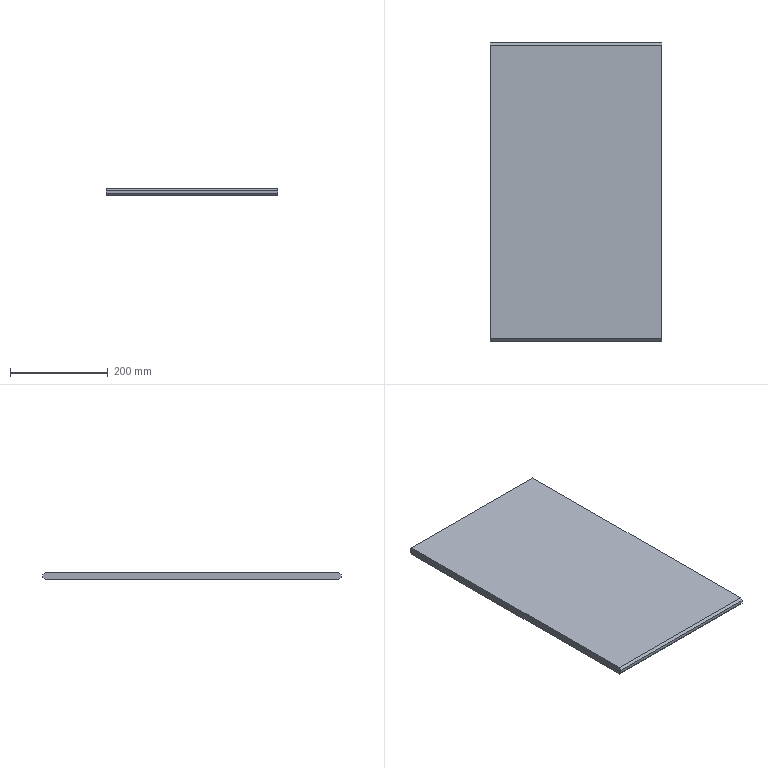Part | SolidWorks | features Chamfer 1, Extrusion 1 | 1 solid | 10 faces | box 350 x 610 x 16 mm | volume 3398500 mm3 | plane 10
STEP:
#1=CARTESIAN_POINT('',(0.,610.,11.));
#2=VERTEX_POINT('',#1);
#3=CARTESIAN_POINT('',(0.,610.,5.));
#4=VERTEX_POINT('',#3);
#5=CARTESIAN_POINT('',(0.,610.,16.));
#6=DIRECTION('',(0.,0.,-1.));
#7=VECTOR('',#6,1000.);
#8=LINE('',#5,#7);
#9=EDGE_CURVE('',#2,#4,#8,.T.);
#10=ORIENTED_EDGE('',*,*,#9,.T.);
#11=CARTESIAN_POINT('',(0.,605.,0.));
#12=VERTEX_POINT('',#11);
#13=CARTESIAN_POINT('',(0.,610.,5.));
#14=DIRECTION('',(0.,-0.7071,-0.7071));
#15=VECTOR('',#14,1000.);
#16=LINE('',#13,#15);
#17=EDGE_CURVE('',#4,#12,#16,.T.);
#18=ORIENTED_EDGE('',*,*,#17,.T.);
#19=CARTESIAN_POINT('',(0.,5.,0.));
#20=VERTEX_POINT('',#19);
#21=CARTESIAN_POINT('',(0.,0.,0.));
#22=DIRECTION('',(0.,-1.,0.));
#23=VECTOR('',#22,1000.);
#24=LINE('',#21,#23);
#25=EDGE_CURVE('',#12,#20,#24,.T.);
#26=ORIENTED_EDGE('',*,*,#25,.T.);
#27=CARTESIAN_POINT('',(0.,0.,5.));
#28=VERTEX_POINT('',#27);
#29=CARTESIAN_POINT('',(0.,0.,5.));
#30=DIRECTION('',(0.,-0.7071,0.7071));
#31=VECTOR('',#30,1000.);
#32=LINE('',#29,#31);
#33=EDGE_CURVE('',#20,#28,#32,.T.);
#34=ORIENTED_EDGE('',*,*,#33,.T.);
#35=CARTESIAN_POINT('',(0.,0.,11.));
#36=VERTEX_POINT('',#35);
#37=CARTESIAN_POINT('',(0.,0.,16.));
#38=DIRECTION('',(0.,0.,-1.));
#39=VECTOR('',#38,1000.);
#40=LINE('',#37,#39);
#41=EDGE_CURVE('',#36,#28,#40,.T.);
#42=ORIENTED_EDGE('',*,*,#41,.F.);
#43=CARTESIAN_POINT('',(0.,5.,16.));
#44=VERTEX_POINT('',#43);
#45=CARTESIAN_POINT('',(0.,5.,16.));
#46=DIRECTION('',(0.,0.7071,0.7071));
#47=VECTOR('',#46,1000.);
#48=LINE('',#45,#47);
#49=EDGE_CURVE('',#36,#44,#48,.T.);
#50=ORIENTED_EDGE('',*,*,#49,.T.);
#51=CARTESIAN_POINT('',(0.,605.,16.));
#52=VERTEX_POINT('',#51);
#53=CARTESIAN_POINT('',(0.,0.,16.));
#54=DIRECTION('',(0.,-1.,0.));
#55=VECTOR('',#54,1000.);
#56=LINE('',#53,#55);
#57=EDGE_CURVE('',#52,#44,#56,.T.);
#58=ORIENTED_EDGE('',*,*,#57,.F.);
#59=CARTESIAN_POINT('',(0.,605.,16.));
#60=DIRECTION('',(0.,0.7071,-0.7071));
#61=VECTOR('',#60,1000.);
#62=LINE('',#59,#61);
#63=EDGE_CURVE('',#52,#2,#62,.T.);
#64=ORIENTED_EDGE('',*,*,#63,.T.);
#65=EDGE_LOOP('',(#10,#18,#26,#34,#42,#50,#58,#64));
#66=FACE_OUTER_BOUND('',#65,.T.);
#67=CARTESIAN_POINT('',(0.,0.,16.));
#68=DIRECTION('',(1.,0.,0.));
#69=DIRECTION('',(0.,0.,-1.));
#70=AXIS2_PLACEMENT_3D('',#67,#68,#69);
#71=PLANE('',#70);
#72=ADVANCED_FACE('',(#66),#71,.F.);
#73=ORIENTED_EDGE('',*,*,#41,.T.);
#74=CARTESIAN_POINT('',(350.,0.,5.));
#75=VERTEX_POINT('',#74);
#76=CARTESIAN_POINT('',(350.,0.,5.));
#77=DIRECTION('',(1.,0.,0.));
#78=VECTOR('',#77,1000.);
#79=LINE('',#76,#78);
#80=EDGE_CURVE('',#28,#75,#79,.T.);
#81=ORIENTED_EDGE('',*,*,#80,.T.);
#82=CARTESIAN_POINT('',(350.,0.,11.));
#83=VERTEX_POINT('',#82);
#84=CARTESIAN_POINT('',(350.,0.,16.));
#85=DIRECTION('',(0.,0.,-1.));
#86=VECTOR('',#85,1000.);
#87=LINE('',#84,#86);
#88=EDGE_CURVE('',#83,#75,#87,.T.);
#89=ORIENTED_EDGE('',*,*,#88,.F.);
#90=CARTESIAN_POINT('',(0.,0.,11.));
#91=DIRECTION('',(-1.,0.,0.));
#92=VECTOR('',#91,1000.);
#93=LINE('',#90,#92);
#94=EDGE_CURVE('',#83,#36,#93,.T.);
#95=ORIENTED_EDGE('',*,*,#94,.T.);
#96=EDGE_LOOP('',(#73,#81,#89,#95));
#97=FACE_OUTER_BOUND('',#96,.T.);
#98=CARTESIAN_POINT('',(0.,0.,16.));
#99=DIRECTION('',(0.,1.,0.));
#100=DIRECTION('',(0.,0.,1.));
#101=AXIS2_PLACEMENT_3D('',#98,#99,#100);
#102=PLANE('',#101);
#103=ADVANCED_FACE('',(#97),#102,.F.);
#104=CARTESIAN_POINT('',(350.,5.,0.));
#105=VERTEX_POINT('',#104);
#106=CARTESIAN_POINT('',(350.,605.,0.));
#107=VERTEX_POINT('',#106);
#108=CARTESIAN_POINT('',(350.,0.,0.));
#109=DIRECTION('',(0.,1.,0.));
#110=VECTOR('',#109,1000.);
#111=LINE('',#108,#110);
#112=EDGE_CURVE('',#105,#107,#111,.T.);
#113=ORIENTED_EDGE('',*,*,#112,.T.);
#114=CARTESIAN_POINT('',(350.,610.,5.));
#115=VERTEX_POINT('',#114);
#116=CARTESIAN_POINT('',(350.,610.,5.));
#117=DIRECTION('',(0.,0.7071,0.7071));
#118=VECTOR('',#117,1000.);
#119=LINE('',#116,#118);
#120=EDGE_CURVE('',#107,#115,#119,.T.);
#121=ORIENTED_EDGE('',*,*,#120,.T.);
#122=CARTESIAN_POINT('',(350.,610.,11.));
#123=VERTEX_POINT('',#122);
#124=CARTESIAN_POINT('',(350.,610.,16.));
#125=DIRECTION('',(0.,0.,-1.));
#126=VECTOR('',#125,1000.);
#127=LINE('',#124,#126);
#128=EDGE_CURVE('',#123,#115,#127,.T.);
#129=ORIENTED_EDGE('',*,*,#128,.F.);
#130=CARTESIAN_POINT('',(350.,605.,16.));
#131=VERTEX_POINT('',#130);
#132=CARTESIAN_POINT('',(350.,605.,16.));
#133=DIRECTION('',(0.,-0.7071,0.7071));
#134=VECTOR('',#133,1000.);
#135=LINE('',#132,#134);
#136=EDGE_CURVE('',#123,#131,#135,.T.);
#137=ORIENTED_EDGE('',*,*,#136,.T.);
#138=CARTESIAN_POINT('',(350.,5.,16.));
#139=VERTEX_POINT('',#138);
#140=CARTESIAN_POINT('',(350.,0.,16.));
#141=DIRECTION('',(0.,1.,0.));
#142=VECTOR('',#141,1000.);
#143=LINE('',#140,#142);
#144=EDGE_CURVE('',#139,#131,#143,.T.);
#145=ORIENTED_EDGE('',*,*,#144,.F.);
#146=CARTESIAN_POINT('',(350.,5.,16.));
#147=DIRECTION('',(0.,-0.7071,-0.7071));
#148=VECTOR('',#147,1000.);
#149=LINE('',#146,#148);
#150=EDGE_CURVE('',#139,#83,#149,.T.);
#151=ORIENTED_EDGE('',*,*,#150,.T.);
#152=ORIENTED_EDGE('',*,*,#88,.T.);
#153=CARTESIAN_POINT('',(350.,0.,5.));
#154=DIRECTION('',(0.,0.7071,-0.7071));
#155=VECTOR('',#154,1000.);
#156=LINE('',#153,#155);
#157=EDGE_CURVE('',#75,#105,#156,.T.);
#158=ORIENTED_EDGE('',*,*,#157,.T.);
#159=EDGE_LOOP('',(#113,#121,#129,#137,#145,#151,#152,#158));
#160=FACE_OUTER_BOUND('',#159,.T.);
#161=CARTESIAN_POINT('',(350.,0.,16.));
#162=DIRECTION('',(-1.,0.,0.));
#163=DIRECTION('',(0.,0.,1.));
#164=AXIS2_PLACEMENT_3D('',#161,#162,#163);
#165=PLANE('',#164);
#166=ADVANCED_FACE('',(#160),#165,.F.);
#167=ORIENTED_EDGE('',*,*,#128,.T.);
#168=CARTESIAN_POINT('',(0.,610.,5.));
#169=DIRECTION('',(-1.,0.,0.));
#170=VECTOR('',#169,1000.);
#171=LINE('',#168,#170);
#172=EDGE_CURVE('',#115,#4,#171,.T.);
#173=ORIENTED_EDGE('',*,*,#172,.T.);
#174=ORIENTED_EDGE('',*,*,#9,.F.);
#175=CARTESIAN_POINT('',(0.,610.,11.));
#176=DIRECTION('',(1.,0.,0.));
#177=VECTOR('',#176,1000.);
#178=LINE('',#175,#177);
#179=EDGE_CURVE('',#2,#123,#178,.T.);
#180=ORIENTED_EDGE('',*,*,#179,.T.);
#181=EDGE_LOOP('',(#167,#173,#174,#180));
#182=FACE_OUTER_BOUND('',#181,.T.);
#183=CARTESIAN_POINT('',(0.,610.,16.));
#184=DIRECTION('',(0.,-1.,0.));
#185=DIRECTION('',(0.,0.,-1.));
#186=AXIS2_PLACEMENT_3D('',#183,#184,#185);
#187=PLANE('',#186);
#188=ADVANCED_FACE('',(#182),#187,.F.);
#189=ORIENTED_EDGE('',*,*,#144,.T.);
#190=CARTESIAN_POINT('',(0.,605.,16.));
#191=DIRECTION('',(-1.,0.,0.));
#192=VECTOR('',#191,1000.);
#193=LINE('',#190,#192);
#194=EDGE_CURVE('',#131,#52,#193,.T.);
#195=ORIENTED_EDGE('',*,*,#194,.T.);
#196=ORIENTED_EDGE('',*,*,#57,.T.);
#197=CARTESIAN_POINT('',(0.,5.,16.));
#198=DIRECTION('',(1.,0.,0.));
#199=VECTOR('',#198,1000.);
#200=LINE('',#197,#199);
#201=EDGE_CURVE('',#44,#139,#200,.T.);
#202=ORIENTED_EDGE('',*,*,#201,.T.);
#203=EDGE_LOOP('',(#189,#195,#196,#202));
#204=FACE_OUTER_BOUND('',#203,.T.);
#205=CARTESIAN_POINT('',(0.,610.,16.));
#206=DIRECTION('',(0.,0.,-1.));
#207=DIRECTION('',(-1.,0.,0.));
#208=AXIS2_PLACEMENT_3D('',#205,#206,#207);
#209=PLANE('',#208);
#210=ADVANCED_FACE('',(#204),#209,.F.);
#211=ORIENTED_EDGE('',*,*,#25,.F.);
#212=CARTESIAN_POINT('',(350.,605.,0.));
#213=DIRECTION('',(1.,0.,0.));
#214=VECTOR('',#213,1000.);
#215=LINE('',#212,#214);
#216=EDGE_CURVE('',#12,#107,#215,.T.);
#217=ORIENTED_EDGE('',*,*,#216,.T.);
#218=ORIENTED_EDGE('',*,*,#112,.F.);
#219=CARTESIAN_POINT('',(0.,5.,0.));
#220=DIRECTION('',(-1.,0.,0.));
#221=VECTOR('',#220,1000.);
#222=LINE('',#219,#221);
#223=EDGE_CURVE('',#105,#20,#222,.T.);
#224=ORIENTED_EDGE('',*,*,#223,.T.);
#225=EDGE_LOOP('',(#211,#217,#218,#224));
#226=FACE_OUTER_BOUND('',#225,.T.);
#227=CARTESIAN_POINT('',(0.,610.,0.));
#228=DIRECTION('',(0.,0.,-1.));
#229=DIRECTION('',(-1.,0.,0.));
#230=AXIS2_PLACEMENT_3D('',#227,#228,#229);
#231=PLANE('',#230);
#232=ADVANCED_FACE('',(#226),#231,.T.);
#233=ORIENTED_EDGE('',*,*,#120,.F.);
#234=ORIENTED_EDGE('',*,*,#216,.F.);
#235=ORIENTED_EDGE('',*,*,#17,.F.);
#236=ORIENTED_EDGE('',*,*,#172,.F.);
#237=EDGE_LOOP('',(#233,#234,#235,#236));
#238=FACE_OUTER_BOUND('',#237,.T.);
#239=CARTESIAN_POINT('',(0.,610.,5.));
#240=DIRECTION('',(0.,0.7071,-0.7071));
#241=DIRECTION('',(0.,0.7071,0.7071));
#242=AXIS2_PLACEMENT_3D('',#239,#240,#241);
#243=PLANE('',#242);
#244=ADVANCED_FACE('',(#238),#243,.T.);
#245=ORIENTED_EDGE('',*,*,#136,.F.);
#246=ORIENTED_EDGE('',*,*,#179,.F.);
#247=ORIENTED_EDGE('',*,*,#63,.F.);
#248=ORIENTED_EDGE('',*,*,#194,.F.);
#249=EDGE_LOOP('',(#245,#246,#247,#248));
#250=FACE_OUTER_BOUND('',#249,.T.);
#251=CARTESIAN_POINT('',(0.,605.,16.));
#252=DIRECTION('',(0.,-0.7071,-0.7071));
#253=DIRECTION('',(0.,0.7071,-0.7071));
#254=AXIS2_PLACEMENT_3D('',#251,#252,#253);
#255=PLANE('',#254);
#256=ADVANCED_FACE('',(#250),#255,.F.);
#257=ORIENTED_EDGE('',*,*,#33,.F.);
#258=ORIENTED_EDGE('',*,*,#223,.F.);
#259=ORIENTED_EDGE('',*,*,#157,.F.);
#260=ORIENTED_EDGE('',*,*,#80,.F.);
#261=EDGE_LOOP('',(#257,#258,#259,#260));
#262=FACE_OUTER_BOUND('',#261,.T.);
#263=CARTESIAN_POINT('',(0.,0.,5.));
#264=DIRECTION('',(0.,-0.7071,-0.7071));
#265=DIRECTION('',(0.,0.7071,-0.7071));
#266=AXIS2_PLACEMENT_3D('',#263,#264,#265);
#267=PLANE('',#266);
#268=ADVANCED_FACE('',(#262),#267,.T.);
#269=ORIENTED_EDGE('',*,*,#49,.F.);
#270=ORIENTED_EDGE('',*,*,#94,.F.);
#271=ORIENTED_EDGE('',*,*,#150,.F.);
#272=ORIENTED_EDGE('',*,*,#201,.F.);
#273=EDGE_LOOP('',(#269,#270,#271,#272));
#274=FACE_OUTER_BOUND('',#273,.T.);
#275=CARTESIAN_POINT('',(0.,5.,16.));
#276=DIRECTION('',(0.,0.7071,-0.7071));
#277=DIRECTION('',(0.,0.7071,0.7071));
#278=AXIS2_PLACEMENT_3D('',#275,#276,#277);
#279=PLANE('',#278);
#280=ADVANCED_FACE('',(#274),#279,.F.);
#281=CLOSED_SHELL('',(#72,#103,#166,#188,#210,#232,#244,#256,#268,#280));
#282=MANIFOLD_SOLID_BREP('',#281);
#283=CARTESIAN_POINT('',(0.,0.,0.));
#284=DIRECTION('',(0.,0.,1.));
#285=DIRECTION('',(1.,0.,0.));
#286=AXIS2_PLACEMENT_3D('',#283,#284,#285);
#287=(LENGTH_UNIT()NAMED_UNIT(*)SI_UNIT(.MILLI.,.METRE.));
#288=UNCERTAINTY_MEASURE_WITH_UNIT(LENGTH_MEASURE(0.00001),#287,'','');
#289=(NAMED_UNIT(*)PLANE_ANGLE_UNIT()SI_UNIT($,.RADIAN.));
#290=(NAMED_UNIT(*)SI_UNIT($,.STERADIAN.)SOLID_ANGLE_UNIT());
#291=(GEOMETRIC_REPRESENTATION_CONTEXT(3)GLOBAL_UNCERTAINTY_ASSIGNED_CONTEXT((#288))GLOBAL_UNIT_ASSIGNED_CONTEXT((#287,#289,#290))REPRESENTATION_CONTEXT('',''));
#292=ADVANCED_BREP_SHAPE_REPRESENTATION('',(#282,#286),#291);